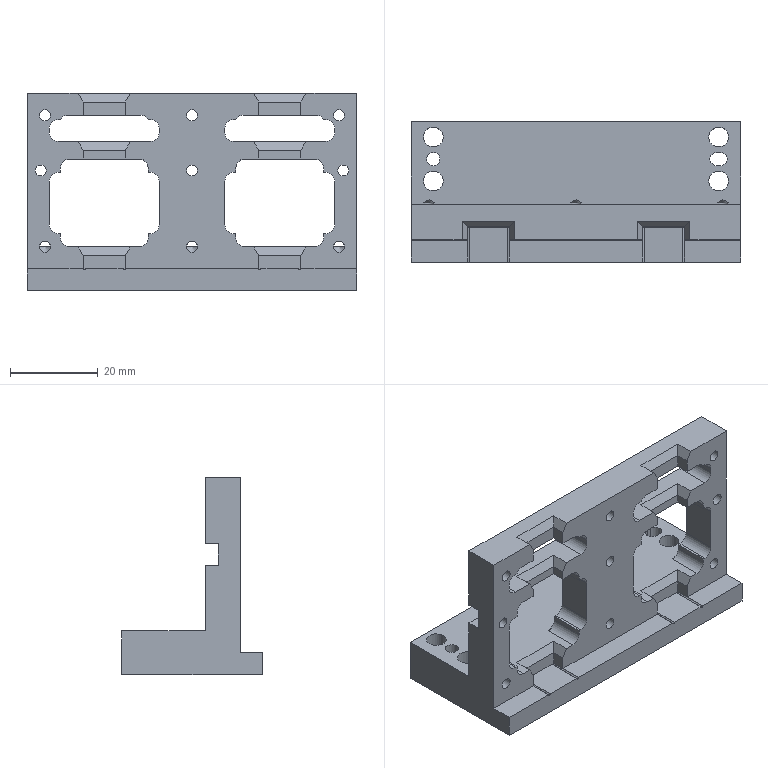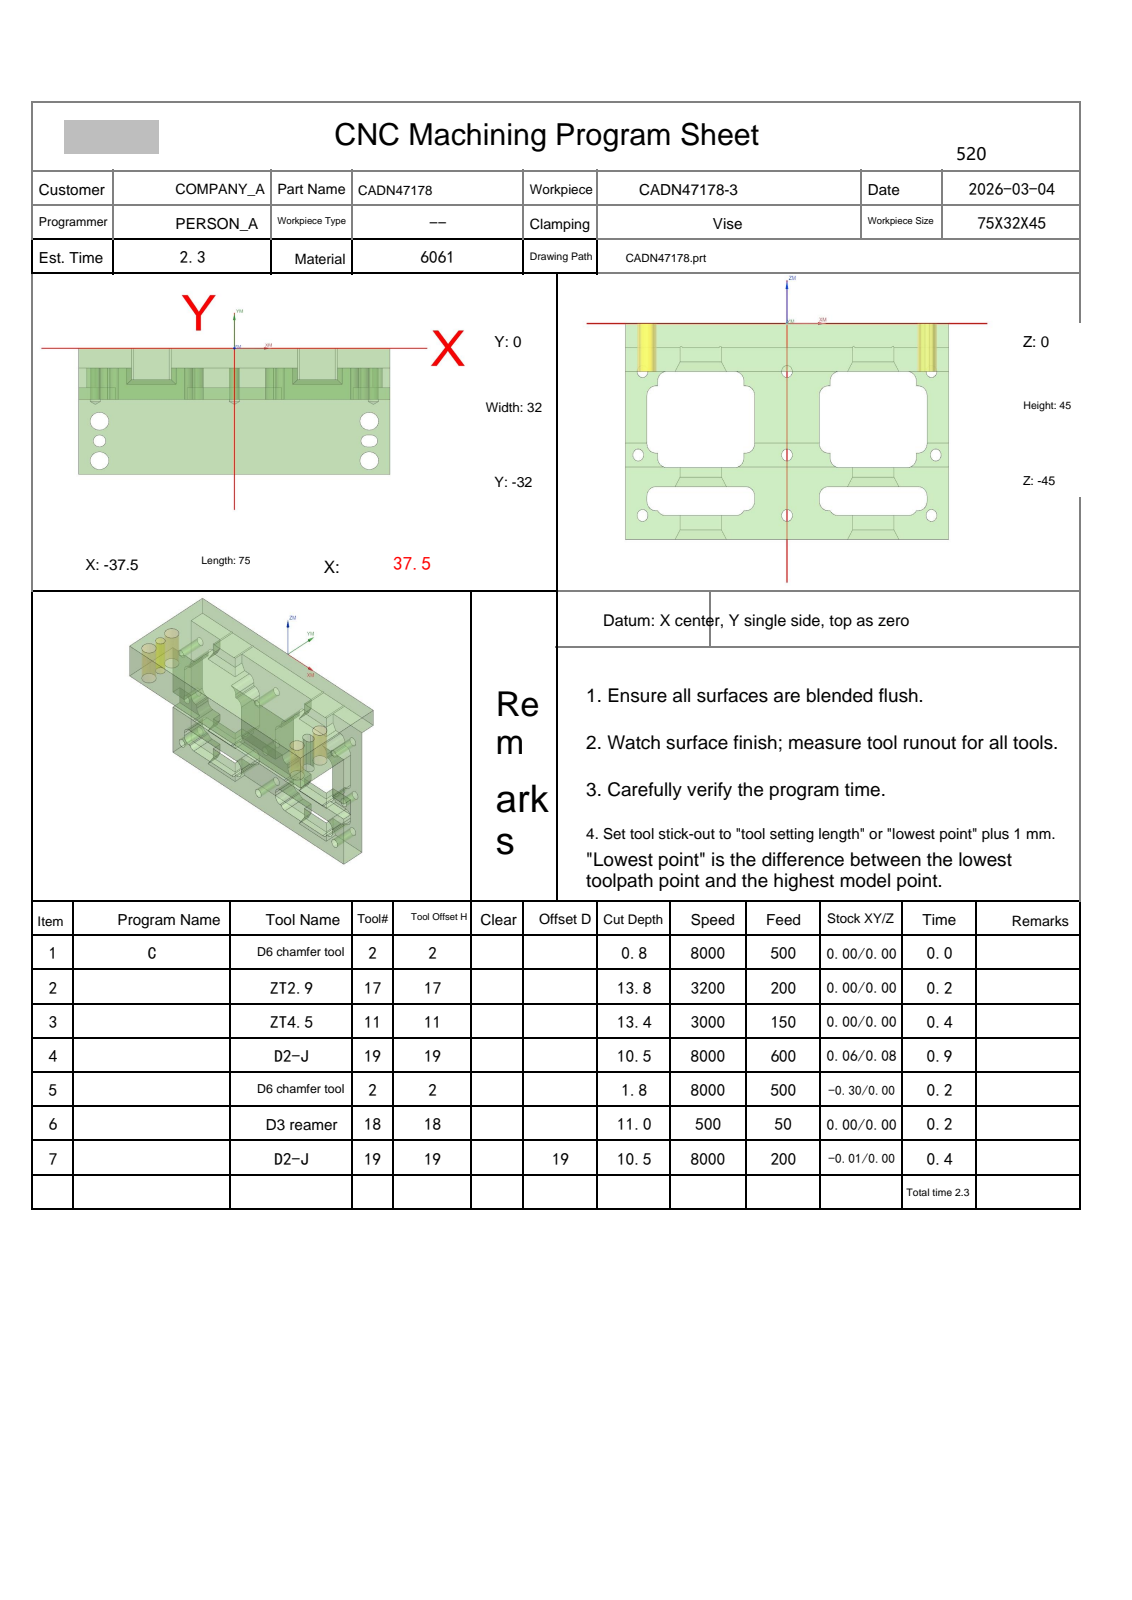NC program | NX | posted by the shop | part box 75 x 32 x 45 mm
Whole program:
%
O0001
(Machine time: 3.72 MIN)
(===Total Tool:5===)
(T2=D6 chamfer tool   D=6.   R=0.   D-  H02 Z=-1.8  )
(T17=ZT2.9  D=2.9  DR_a=120 D-  H17 Z=-13.84)
(T11=ZT4.5  D=4.5  DR_a=118 D-  H11 Z=-13.35)
(T19=D2-J   D=2.   R=0.   D-  H19 Z=-10.5 )
(T18=D3 reamer   D=3.   DR_a=180 D-  H18 Z=-11.  )
G80 G90 G17 G49 G40
G91 G28 Z0
M01
N1 T02 M06
(D6 chamfer tool  D=6. R=0. H=02 ce=0.00 di=0.00)
G00 G90 G54 X-32.5 Y-28.5 M03 S8000
G43 H02 Z30.
M08
G98 G81 X-32.5 Y-28.5 Z-.8 R1. F500.
Y-23.5
Y-18.5
X32.5
Y-28.5
G80
G00 Z30.
G00 G90 X32. Y-23.5 M03 S8000
Z30.
G98 G81 X32. Y-23.5 Z-.8 R1. F500.
G80
G00 Z30.
G91 G28 Z0.0
M05
M09
G91 G28 Z0.0
M01
N2 T17 M06
(ZT2.9 D=2.9 DR_a=120 H=17)
G00 G90 G54 X-32.5 Y-23.5 M03 S3200
G43 H17 Z30.
M08
G98 G83 X-32.5 Y-23.5 Z-13.837 R1. F200. Q2.
G80
G00 Z30.
G00 G90 X32. Y-23.5 M03 S3200
Z30.
G98 G83 X32. Y-23.5 Z-13.837 R1. F200. Q2.
G80
G00 Z30.
G91 G28 Z0.0
M05
M09
G91 G28 Z0.0
M01
N3 T11 M06
(ZT4.5 D=4.5 DR_a=118 H=11)
G00 G90 G54 X-32.5 Y-28.5 M03 S3000
G43 H11 Z30.
M08
G98 G83 X-32.5 Y-28.5 Z-13.352 R1. F150. Q3.
Y-18.5
X32.5
Y-28.5
G80
G00 Z30.
G91 G28 Z0.0
M05
M09
G91 G28 Z0.0
M01
N4 T19 M06
(D2-J  D=2. R=0. H=19 ce=0.06 di=0.08)
G00 G90 G54 X31.56 Y-23.583 M03 S8000
G43 H19 Z30.
M08
Z.8
G01 Y-23.665 Z.796 F600.
X31.835 Y-23.94 Z.775
X33.165 Z.706
X33.44 Y-23.665 Z.685
Y-23.335 Z.668
X33.165 Y-23.06 Z.648
X31.835 Z.578
X31.56 Y-23.335 Z.557
Y-23.665 Z.54
X31.835 Y-23.94 Z.52
X33.165 Z.45
X33.44 Y-23.665 Z.43
Y-23.335 Z.412
X33.165 Y-23.06 Z.392
X31.835 Z.322
X31.56 Y-23.335 Z.302
Y-23.665 Z.285
X31.835 Y-23.94 Z.264
X33.165 Z.194
X33.44 Y-23.665 Z.174
Y-23.335 Z.157
X33.165 Y-23.06 Z.136
X31.835 Z.067
X31.56 Y-23.335 Z.046
Y-23.665 Z.029
X31.835 Y-23.94 Z.009
X32. Z0.0
X33. Z-.021
G03 X33.44 Y-23.5 Z-.035 I0.0 J.44
X33. Y-23.06 Z-.05 I-.44 J0.0
G01 X32. Z-.07
G03 X31.56 Y-23.5 Z-.085 I0.0 J-.44
X32. Y-23.94 Z-.099 I.44 J0.0
G01 X33. Z-.12
G03 X33.44 Y-23.5 Z-.134 I0.0 J.44
X33. Y-23.06 Z-.149 I-.44 J0.0
G01 X32. Z-.169
G03 X31.56 Y-23.5 Z-.184 I0.0 J-.44
X32. Y-23.94 Z-.198 I.44 J0.0
G01 X33. Z-.219
G03 X33.44 Y-23.5 Z-.233 I0.0 J.44
X33. Y-23.06 Z-.248 I-.44 J0.0
G01 X32. Z-.268
G03 X31.56 Y-23.5 Z-.283 I0.0 J-.44
X32. Y-23.94 Z-.297 I.44 J0.0
G01 X33. Z-.318
G03 X33.44 Y-23.5 Z-.332 I0.0 J.44
X33. Y-23.06 Z-.347 I-.44 J0.0
G01 X32. Z-.367
G03 X31.56 Y-23.5 Z-.382 I0.0 J-.44
X32. Y-23.94 Z-.396 I.44 J0.0
G01 X33. Z-.417
G03 X33.44 Y-23.5 Z-.431 I0.0 J.44
X33. Y-23.06 Z-.446 I-.44 J0.0
G01 X32. Z-.467
G03 X31.56 Y-23.5 Z-.481 I0.0 J-.44
X32. Y-23.94 Z-.495 I.44 J0.0
G01 X33. Z-.516
G03 X33.44 Y-23.5 Z-.53 I0.0 J.44
X33. Y-23.06 Z-.545 I-.44 J0.0
G01 X32. Z-.566
G03 X31.56 Y-23.5 Z-.58 I0.0 J-.44
X32. Y-23.94 Z-.594 I.44 J0.0
G01 X33. Z-.615
G03 X33.44 Y-23.5 Z-.629 I0.0 J.44
X33. Y-23.06 Z-.644 I-.44 J0.0
G01 X32. Z-.665
G03 X31.56 Y-23.5 Z-.679 I0.0 J-.44
X32. Y-23.94 Z-.693 I.44 J0.0
G01 X33. Z-.714
G03 X33.44 Y-23.5 Z-.729 I0.0 J.44
X33. Y-23.06 Z-.743 I-.44 J0.0
G01 X32. Z-.764
G03 X31.56 Y-23.5 Z-.778 I0.0 J-.44
X32. Y-23.94 Z-.792 I.44 J0.0
G01 X33. Z-.813
G03 X33.44 Y-23.5 Z-.828 I0.0 J.44
X33. Y-23.06 Z-.842 I-.44 J0.0
G01 X32. Z-.863
G03 X31.56 Y-23.5 Z-.877 I0.0 J-.44
X32. Y-23.94 Z-.892 I.44 J0.0
G01 X33. Z-.912
G03 X33.44 Y-23.5 Z-.927 I0.0 J.44
X33. Y-23.06 Z-.941 I-.44 J0.0
G01 X32. Z-.962
G03 X31.56 Y-23.5 Z-.976 I0.0 J-.44
X32. Y-23.94 Z-.991 I.44 J0.0
G01 X33. Z-1.011
G03 X33.44 Y-23.5 Z-1.026 I0.0 J.44
X33. Y-23.06 Z-1.04 I-.44 J0.0
G01 X32. Z-1.061
G03 X31.56 Y-23.5 Z-1.075 I0.0 J-.44
X32. Y-23.94 Z-1.09 I.44 J0.0
G01 X33. Z-1.11
G03 X33.44 Y-23.5 Z-1.125 I0.0 J.44
X33. Y-23.06 Z-1.139 I-.44 J0.0
G01 X32. Z-1.16
G03 X31.56 Y-23.5 Z-1.174 I0.0 J-.44
X32. Y-23.94 Z-1.189 I.44 J0.0
G01 X33. Z-1.209
G03 X33.44 Y-23.5 Z-1.224 I0.0 J.44
X33. Y-23.06 Z-1.238 I-.44 J0.0
G01 X32. Z-1.259
G03 X31.56 Y-23.5 Z-1.273 I0.0 J-.44
X32. Y-23.94 Z-1.288 I.44 J0.0
G01 X33. Z-1.309
G03 X33.44 Y-23.5 Z-1.323 I0.0 J.44
X33. Y-23.06 Z-1.337 I-.44 J0.0
G01 X32. Z-1.358
G03 X31.56 Y-23.5 Z-1.372 I0.0 J-.44
X32. Y-23.94 Z-1.387 I.44 J0.0
G01 X33. Z-1.408
G03 X33.44 Y-23.5 Z-1.422 I0.0 J.44
X33. Y-23.06 Z-1.436 I-.44 J0.0
G01 X32. Z-1.457
G03 X31.56 Y-23.5 Z-1.471 I0.0 J-.44
X32. Y-23.94 Z-1.486 I.44 J0.0
G01 X33. Z-1.507
G03 X33.44 Y-23.5 Z-1.521 I0.0 J.44
X33. Y-23.06 Z-1.535 I-.44 J0.0
G01 X32. Z-1.556
G03 X31.56 Y-23.5 Z-1.571 I0.0 J-.44
X32. Y-23.94 Z-1.585 I.44 J0.0
G01 X33. Z-1.606
G03 X33.44 Y-23.5 Z-1.62 I0.0 J.44
X33. Y-23.06 Z-1.634 I-.44 J0.0
G01 X32. Z-1.655
G03 X31.56 Y-23.5 Z-1.67 I0.0 J-.44
X32. Y-23.94 Z-1.684 I.44 J0.0
G01 X33. Z-1.705
G03 X33.44 Y-23.5 Z-1.719 I0.0 J.44
X33. Y-23.06 Z-1.733 I-.44 J0.0
G01 X32. Z-1.754
G03 X31.56 Y-23.5 Z-1.769 I0.0 J-.44
X32. Y-23.94 Z-1.783 I.44 J0.0
G01 X33. Z-1.804
G03 X33.44 Y-23.5 Z-1.818 I0.0 J.44
X33. Y-23.06 Z-1.833 I-.44 J0.0
G01 X32. Z-1.853
G03 X31.56 Y-23.5 Z-1.868 I0.0 J-.44
X32. Y-23.94 Z-1.882 I.44 J0.0
G01 X33. Z-1.903
G03 X33.44 Y-23.5 Z-1.917 I0.0 J.44
X33. Y-23.06 Z-1.932 I-.44 J0.0
G01 X32. Z-1.952
G03 X31.56 Y-23.5 Z-1.967 I0.0 J-.44
X32. Y-23.94 Z-1.981 I.44 J0.0
G01 X33. Z-2.002
G03 X33.44 Y-23.5 Z-2.016 I0.0 J.44
X33. Y-23.06 Z-2.031 I-.44 J0.0
G01 X32. Z-2.051
G03 X31.56 Y-23.5 Z-2.066 I0.0 J-.44
X32. Y-23.94 Z-2.08 I.44 J0.0
G01 X33. Z-2.101
G03 X33.44 Y-23.5 Z-2.115 I0.0 J.44
X33. Y-23.06 Z-2.13 I-.44 J0.0
G01 X32. Z-2.151
G03 X31.56 Y-23.5 Z-2.165 I0.0 J-.44
X32. Y-23.94 Z-2.179 I.44 J0.0
G01 X33. Z-2.2
G03 X33.44 Y-23.5 Z-2.214 I0.0 J.44
X33. Y-23.06 Z-2.229 I-.44 J0.0
G01 X32. Z-2.25
G03 X31.56 Y-23.5 Z-2.264 I0.0 J-.44
X32. Y-23.94 Z-2.278 I.44 J0.0
G01 X33. Z-2.299
G03 X33.44 Y-23.5 Z-2.313 I0.0 J.44
X33. Y-23.06 Z-2.328 I-.44 J0.0
G01 X32. Z-2.349
G03 X31.56 Y-23.5 Z-2.363 I0.0 J-.44
X32. Y-23.94 Z-2.377 I.44 J0.0
G01 X33. Z-2.398
G03 X33.44 Y-23.5 Z-2.413 I0.0 J.44
X33. Y-23.06 Z-2.427 I-.44 J0.0
G01 X32. Z-2.448
G03 X31.56 Y-23.5 Z-2.462 I0.0 J-.44
X32. Y-23.94 Z-2.476 I.44 J0.0
G01 X33. Z-2.497
G03 X33.44 Y-23.5 Z-2.512 I0.0 J.44
X33. Y-23.06 Z-2.526 I-.44 J0.0
G01 X32. Z-2.547
G03 X31.56 Y-23.5 Z-2.561 I0.0 J-.44
X32. Y-23.94 Z-2.575 I.44 J0.0
G01 X33. Z-2.596
G03 X33.44 Y-23.5 Z-2.611 I0.0 J.44
X33. Y-23.06 Z-2.625 I-.44 J0.0
G01 X32. Z-2.646
G03 X31.56 Y-23.5 Z-2.66 I0.0 J-.44
X32. Y-23.94 Z-2.675 I.44 J0.0
G01 X33. Z-2.695
G03 X33.44 Y-23.5 Z-2.71 I0.0 J.44
X33. Y-23.06 Z-2.724 I-.44 J0.0
G01 X32. Z-2.745
G03 X31.56 Y-23.5 Z-2.759 I0.0 J-.44
X32. Y-23.94 Z-2.774 I.44 J0.0
G01 X33. Z-2.794
G03 X33.44 Y-23.5 Z-2.809 I0.0 J.44
X33. Y-23.06 Z-2.823 I-.44 J0.0
G01 X32. Z-2.844
G03 X31.56 Y-23.5 Z-2.858 I0.0 J-.44
X32. Y-23.94 Z-2.873 I.44 J0.0
G01 X33. Z-2.893
G03 X33.44 Y-23.5 Z-2.908 I0.0 J.44
X33. Y-23.06 Z-2.922 I-.44 J0.0
G01 X32. Z-2.943
G03 X31.56 Y-23.5 Z-2.957 I0.0 J-.44
X32. Y-23.94 Z-2.972 I.44 J0.0
G01 X33. Z-2.992
G03 X33.44 Y-23.5 Z-3.007 I0.0 J.44
X33. Y-23.06 Z-3.021 I-.44 J0.0
G01 X32. Z-3.042
G03 X31.56 Y-23.5 Z-3.056 I0.0 J-.44
X32. Y-23.94 Z-3.071 I.44 J0.0
G01 X33. Z-3.092
G03 X33.44 Y-23.5 Z-3.106 I0.0 J.44
X33. Y-23.06 Z-3.12 I-.44 J0.0
G01 X32. Z-3.141
G03 X31.56 Y-23.5 Z-3.155 I0.0 J-.44
X32. Y-23.94 Z-3.17 I.44 J0.0
G01 X33. Z-3.191
G03 X33.44 Y-23.5 Z-3.205 I0.0 J.44
X33. Y-23.06 Z-3.219 I-.44 J0.0
G01 X32. Z-3.24
G03 X31.56 Y-23.5 Z-3.254 I0.0 J-.44
X32. Y-23.94 Z-3.269 I.44 J0.0
G01 X33. Z-3.29
G03 X33.44 Y-23.5 Z-3.304 I0.0 J.44
X33. Y-23.06 Z-3.318 I-.44 J0.0
G01 X32. Z-3.339
G03 X31.56 Y-23.5 Z-3.354 I0.0 J-.44
X32. Y-23.94 Z-3.368 I.44 J0.0
G01 X33. Z-3.389
G03 X33.44 Y-23.5 Z-3.403 I0.0 J.44
X33. Y-23.06 Z-3.417 I-.44 J0.0
G01 X32. Z-3.438
G03 X31.56 Y-23.5 Z-3.453 I0.0 J-.44
X32. Y-23.94 Z-3.467 I.44 J0.0
G01 X33. Z-3.488
G03 X33.44 Y-23.5 Z-3.502 I0.0 J.44
X33. Y-23.06 Z-3.517 I-.44 J0.0
G01 X32. Z-3.537
G03 X31.56 Y-23.5 Z-3.552 I0.0 J-.44
X32. Y-23.94 Z-3.566 I.44 J0.0
G01 X33. Z-3.587
G03 X33.44 Y-23.5 Z-3.601 I0.0 J.44
X33. Y-23.06 Z-3.616 I-.44 J0.0
G01 X32. Z-3.636
G03 X31.56 Y-23.5 Z-3.651 I0.0 J-.44
X32. Y-23.94 Z-3.665 I.44 J0.0
G01 X33. Z-3.686
G03 X33.44 Y-23.5 Z-3.7 I0.0 J.44
X33. Y-23.06 Z-3.715 I-.44 J0.0
G01 X32. Z-3.735
G03 X31.56 Y-23.5 Z-3.75 I0.0 J-.44
X32. Y-23.94 Z-3.764 I.44 J0.0
G01 X33. Z-3.785
G03 X33.44 Y-23.5 Z-3.799 I0.0 J.44
X33. Y-23.06 Z-3.814 I-.44 J0.0
G01 X32. Z-3.834
G03 X31.56 Y-23.5 Z-3.849 I0.0 J-.44
X32. Y-23.94 Z-3.863 I.44 J0.0
G01 X33. Z-3.884
G03 X33.44 Y-23.5 Z-3.898 I0.0 J.44
X33. Y-23.06 Z-3.913 I-.44 J0.0
G01 X32. Z-3.934
G03 X31.56 Y-23.5 Z-3.948 I0.0 J-.44
X32. Y-23.94 Z-3.962 I.44 J0.0
G01 X33. Z-3.983
G03 X33.44 Y-23.5 Z-3.997 I0.0 J.44
X33. Y-23.06 Z-4.012 I-.44 J0.0
G01 X32. Z-4.033
G03 X31.56 Y-23.5 Z-4.047 I0.0 J-.44
X32. Y-23.94 Z-4.061 I.44 J0.0
G01 X33. Z-4.082
G03 X33.44 Y-23.5 Z-4.096 I0.0 J.44
X33. Y-23.06 Z-4.111 I-.44 J0.0
G01 X32. Z-4.132
G03 X31.56 Y-23.5 Z-4.146 I0.0 J-.44
X32. Y-23.94 Z-4.16 I.44 J0.0
G01 X33. Z-4.181
G03 X33.44 Y-23.5 Z-4.196 I0.0 J.44
X33. Y-23.06 Z-4.21 I-.44 J0.0
G01 X32. Z-4.231
G03 X31.56 Y-23.5 Z-4.245 I0.0 J-.44
X32. Y-23.94 Z-4.259 I.44 J0.0
G01 X33. Z-4.28
G03 X33.44 Y-23.5 Z-4.295 I0.0 J.44
X33. Y-23.06 Z-4.309 I-.44 J0.0
G01 X32. Z-4.33
G03 X31.56 Y-23.5 Z-4.344 I0.0 J-.44
X32. Y-23.94 Z-4.358 I.44 J0.0
G01 X33. Z-4.379
G03 X33.44 Y-23.5 Z-4.394 I0.0 J.44
X33. Y-23.06 Z-4.408 I-.44 J0.0
G01 X32. Z-4.429
G03 X31.56 Y-23.5 Z-4.443 I0.0 J-.44
X32. Y-23.94 Z-4.458 I.44 J0.0
G01 X33. Z-4.478
G03 X33.44 Y-23.5 Z-4.493 I0.0 J.44
X33. Y-23.06 Z-4.507 I-.44 J0.0
G01 X32. Z-4.528
G03 X31.56 Y-23.5 Z-4.542 I0.0 J-.44
X32. Y-23.94 Z-4.557 I.44 J0.0
G01 X33. Z-4.577
G03 X33.44 Y-23.5 Z-4.592 I0.0 J.44
X33. Y-23.06 Z-4.606 I-.44 J0.0
G01 X32. Z-4.627
G03 X31.56 Y-23.5 Z-4.641 I0.0 J-.44
X32. Y-23.94 Z-4.656 I.44 J0.0
G01 X33. Z-4.676
G03 X33.44 Y-23.5 Z-4.691 I0.0 J.44
X33. Y-23.06 Z-4.705 I-.44 J0.0
G01 X32. Z-4.726
G03 X31.56 Y-23.5 Z-4.74 I0.0 J-.44
X32. Y-23.94 Z-4.755 I.44 J0.0
G01 X33. Z-4.776
G03 X33.44 Y-23.5 Z-4.79 I0.0 J.44
X33. Y-23.06 Z-4.804 I-.44 J0.0
G01 X32. Z-4.825
G03 X31.56 Y-23.5 Z-4.839 I0.0 J-.44
X32. Y-23.94 Z-4.854 I.44 J0.0
G01 X33. Z-4.875
G03 X33.44 Y-23.5 Z-4.889 I0.0 J.44
X33. Y-23.06 Z-4.903 I-.44 J0.0
G01 X32. Z-4.924
G03 X31.56 Y-23.5 Z-4.938 I0.0 J-.44
X32. Y-23.94 Z-4.953 I.44 J0.0
G01 X33. Z-4.974
G03 X33.44 Y-23.5 Z-4.988 I0.0 J.44
X33. Y-23.06 Z-5.002 I-.44 J0.0
G01 X32. Z-5.023
G03 X31.56 Y-23.5 Z-5.038 I0.0 J-.44
X32. Y-23.94 Z-5.052 I.44 J0.0
G01 X33. Z-5.073
G03 X33.44 Y-23.5 Z-5.087 I0.0 J.44
X33. Y-23.06 Z-5.101 I-.44 J0.0
G01 X32. Z-5.122
G03 X31.56 Y-23.5 Z-5.137 I0.0 J-.44
X32. Y-23.94 Z-5.151 I.44 J0.0
G01 X33. Z-5.172
G03 X33.44 Y-23.5 Z-5.186 I0.0 J.44
X33. Y-23.06 Z-5.2 I-.44 J0.0
G01 X32. Z-5.221
G03 X31.56 Y-23.5 Z-5.236 I0.0 J-.44
X32. Y-23.94 Z-5.25 I.44 J0.0
G01 X33. Z-5.271
G03 X33.44 Y-23.5 Z-5.285 I0.0 J.44
X33. Y-23.06 Z-5.3 I-.44 J0.0
G01 X32. Z-5.32
G03 X31.56 Y-23.5 Z-5.335 I0.0 J-.44
X32. Y-23.94 Z-5.349 I.44 J0.0
G01 X33. Z-5.37
G03 X33.44 Y-23.5 Z-5.384 I0.0 J.44
X33. Y-23.06 Z-5.399 I-.44 J0.0
G01 X32. Z-5.419
G03 X31.56 Y-23.5 Z-5.434 I0.0 J-.44
X32. Y-23.94 Z-5.448 I.44 J0.0
G01 X33. Z-5.469
G03 X33.44 Y-23.5 Z-5.483 I0.0 J.44
X33. Y-23.06 Z-5.498 I-.44 J0.0
G01 X32. Z-5.518
G03 X31.56 Y-23.5 Z-5.533 I0.0 J-.44
X32. Y-23.94 Z-5.547 I.44 J0.0
G01 X33. Z-5.568
G03 X33.44 Y-23.5 Z-5.582 I0.0 J.44
X33. Y-23.06 Z-5.597 I-.44 J0.0
G01 X32. Z-5.617
G03 X31.56 Y-23.5 Z-5.632 I0.0 J-.44
X32. Y-23.94 Z-5.646 I.44 J0.0
G01 X33. Z-5.667
G03 X33.44 Y-23.5 Z-5.681 I0.0 J.44
X33. Y-23.06 Z-5.696 I-.44 J0.0
G01 X32. Z-5.717
G03 X31.56 Y-23.5 Z-5.731 I0.0 J-.44
X32. Y-23.94 Z-5.745 I.44 J0.0
G01 X33. Z-5.766
G03 X33.44 Y-23.5 Z-5.78 I0.0 J.44
X33. Y-23.06 Z-5.795 I-.44 J0.0
G01 X32. Z-5.816
G03 X31.56 Y-23.5 Z-5.83 I0.0 J-.44
X32. Y-23.94 Z-5.844 I.44 J0.0
G01 X33. Z-5.865
G03 X33.44 Y-23.5 Z-5.879 I0.0 J.44
X33. Y-23.06 Z-5.894 I-.44 J0.0
G01 X32. Z-5.915
G03 X31.56 Y-23.5 Z-5.929 I0.0 J-.44
X32. Y-23.94 Z-5.943 I.44 J0.0
G01 X33. Z-5.964
G03 X33.44 Y-23.5 Z-5.979 I0.0 J.44
X33. Y-23.06 Z-5.993 I-.44 J0.0
G01 X32. Z-6.014
G03 X31.56 Y-23.5 Z-6.028 I0.0 J-.44
X32. Y-23.94 Z-6.042 I.44 J0.0
G01 X33. Z-6.063
G03 X33.44 Y-23.5 Z-6.078 I0.0 J.44
X33. Y-23.06 Z-6.092 I-.44 J0.0
G01 X32. Z-6.113
G03 X31.56 Y-23.5 Z-6.127 I0.0 J-.44
X32. Y-23.94 Z-6.142 I.44 J0.0
G01 X33. Z-6.162
G03 X33.44 Y-23.5 Z-6.177 I0.0 J.44
X33. Y-23.06 Z-6.191 I-.44 J0.0
G01 X32. Z-6.212
G03 X31.56 Y-23.5 Z-6.226 I0.0 J-.44
X32. Y-23.94 Z-6.241 I.44 J0.0
G01 X33. Z-6.261
G03 X33.44 Y-23.5 Z-6.276 I0.0 J.44
X33. Y-23.06 Z-6.29 I-.44 J0.0
G01 X32. Z-6.311
G03 X31.56 Y-23.5 Z-6.325 I0.0 J-.44
X32. Y-23.94 Z-6.34 I.44 J0.0
G01 X33. Z-6.36
G03 X33.44 Y-23.5 Z-6.375 I0.0 J.44
X33. Y-23.06 Z-6.389 I-.44 J0.0
G01 X32. Z-6.41
G03 X31.56 Y-23.5 Z-6.424 I0.0 J-.44
X32. Y-23.94 Z-6.439 I.44 J0.0
G01 X33. Z-6.459
G03 X33.44 Y-23.5 Z-6.474 I0.0 J.44
X33. Y-23.06 Z-6.488 I-.44 J0.0
G01 X32. Z-6.509
G03 X31.56 Y-23.5 Z-6.523 I0.0 J-.44
X32. Y-23.94 Z-6.538 I.44 J0.0
G01 X33. Z-6.559
G03 X33.44 Y-23.5 Z-6.573 I0.0 J.44
X33. Y-23.06 Z-6.587 I-.44 J0.0
G01 X32. Z-6.608
G03 X31.56 Y-23.5 Z-6.622 I0.0 J-.44
X32. Y-23.94 Z-6.637 I.44 J0.0
G01 X33. Z-6.658
G03 X33.44 Y-23.5 Z-6.672 I0.0 J.44
X33. Y-23.06 Z-6.686 I-.44 J0.0
G01 X32. Z-6.707
G03 X31.56 Y-23.5 Z-6.721 I0.0 J-.44
X32. Y-23.94 Z-6.736 I.44 J0.0
G01 X33. Z-6.757
G03 X33.44 Y-23.5 Z-6.771 I0.0 J.44
X33. Y-23.06 Z-6.785 I-.44 J0.0
G01 X32. Z-6.806
G03 X31.56 Y-23.5 Z-6.821 I0.0 J-.44
X32. Y-23.94 Z-6.835 I.44 J0.0
G01 X33. Z-6.856
G03 X33.44 Y-23.5 Z-6.87 I0.0 J.44
X33. Y-23.06 Z-6.884 I-.44 J0.0
G01 X32. Z-6.905
G03 X31.56 Y-23.5 Z-6.92 I0.0 J-.44
X32. Y-23.94 Z-6.934 I.44 J0.0
G01 X33. Z-6.955
G03 X33.44 Y-23.5 Z-6.969 I0.0 J.44
X33. Y-23.06 Z-6.983 I-.44 J0.0
G01 X32. Z-7.004
G03 X31.56 Y-23.5 Z-7.019 I0.0 J-.44
X32. Y-23.94 Z-7.033 I.44 J0.0
G01 X33. Z-7.054
G03 X33.44 Y-23.5 Z-7.068 I0.0 J.44
X33. Y-23.06 Z-7.083 I-.44 J0.0
G01 X32. Z-7.103
G03 X31.56 Y-23.5 Z-7.118 I0.0 J-.44
X32. Y-23.94 Z-7.132 I.44 J0.0
G01 X33. Z-7.153
G03 X33.44 Y-23.5 Z-7.167 I0.0 J.44
X33. Y-23.06 Z-7.182 I-.44 J0.0
G01 X32. Z-7.202
G03 X31.56 Y-23.5 Z-7.217 I0.0 J-.44
X32. Y-23.94 Z-7.231 I.44 J0.0
G01 X33. Z-7.252
G03 X33.44 Y-23.5 Z-7.266 I0.0 J.44
X33. Y-23.06 Z-7.281 I-.44 J0.0
G01 X32. Z-7.301
G03 X31.56 Y-23.5 Z-7.316 I0.0 J-.44
X32. Y-23.94 Z-7.33 I.44 J0.0
G01 X33. Z-7.351
G03 X33.44 Y-23.5 Z-7.365 I0.0 J.44
X33. Y-23.06 Z-7.38 I-.44 J0.0
G01 X32. Z-7.401
G03 X31.56 Y-23.5 Z-7.415 I0.0 J-.44
X32. Y-23.94 Z-7.429 I.44 J0.0
G01 X33. Z-7.45
G03 X33.44 Y-23.5 Z-7.464 I0.0 J.44
X33. Y-23.06 Z-7.479 I-.44 J0.0
G01 X32. Z-7.5
G03 X31.56 Y-23.5 Z-7.514 I0.0 J-.44
X32. Y-23.94 Z-7.528 I.44 J0.0
G01 X33. Z-7.549
G03 X33.44 Y-23.5 Z-7.563 I0.0 J.44
X33. Y-23.06 Z-7.578 I-.44 J0.0
G01 X32. Z-7.599
G03 X31.56 Y-23.5 Z-7.613 I0.0 J-.44
X32. Y-23.94 Z-7.627 I.44 J0.0
G01 X33. Z-7.648
G03 X33.44 Y-23.5 Z-7.663 I0.0 J.44
X33. Y-23.06 Z-7.677 I-.44 J0.0
G01 X32. Z-7.698
G03 X31.56 Y-23.5 Z-7.712 I0.0 J-.44
X32. Y-23.94 Z-7.726 I.44 J0.0
G01 X33. Z-7.747
G03 X33.44 Y-23.5 Z-7.762 I0.0 J.44
X33. Y-23.06 Z-7.776 I-.44 J0.0
G01 X32. Z-7.797
G03 X31.56 Y-23.5 Z-7.811 I0.0 J-.44
X32. Y-23.94 Z-7.825 I.44 J0.0
G01 X33. Z-7.846
G03 X33.44 Y-23.5 Z-7.861 I0.0 J.44
X33. Y-23.06 Z-7.875 I-.44 J0.0
G01 X32. Z-7.896
G03 X31.56 Y-23.5 Z-7.91 I0.0 J-.44
X32. Y-23.94 Z-7.925 I.44 J0.0
G01 X33. Z-7.945
G03 X33.44 Y-23.5 Z-7.96 I0.0 J.44
X33. Y-23.06 Z-7.974 I-.44 J0.0
G01 X32. Z-7.995
G03 X31.56 Y-23.5 Z-8.009 I0.0 J-.44
X32. Y-23.94 Z-8.024 I.44 J0.0
G01 X33. Z-8.044
G03 X33.44 Y-23.5 Z-8.059 I0.0 J.44
X33. Y-23.06 Z-8.073 I-.44 J0.0
G01 X32. Z-8.094
G03 X31.56 Y-23.5 Z-8.108 I0.0 J-.44
X32. Y-23.94 Z-8.123 I.44 J0.0
G01 X33. Z-8.143
G03 X33.44 Y-23.5 Z-8.158 I0.0 J.44
X33. Y-23.06 Z-8.172 I-.44 J0.0
G01 X32. Z-8.193
G03 X31.56 Y-23.5 Z-8.207 I0.0 J-.44
X32. Y-23.94 Z-8.222 I.44 J0.0
G01 X33. Z-8.242
G03 X33.44 Y-23.5 Z-8.257 I0.0 J.44
X33. Y-23.06 Z-8.271 I-.44 J0.0
G01 X32. Z-8.292
G03 X31.56 Y-23.5 Z-8.306 I0.0 J-.44
X32. Y-23.94 Z-8.321 I.44 J0.0
G01 X33. Z-8.342
G03 X33.44 Y-23.5 Z-8.356 I0.0 J.44
X33. Y-23.06 Z-8.37 I-.44 J0.0
G01 X32. Z-8.391
G03 X31.56 Y-23.5 Z-8.405 I0.0 J-.44
X32. Y-23.94 Z-8.42 I.44 J0.0
G01 X33. Z-8.441
G03 X33.44 Y-23.5 Z-8.455 I0.0 J.44
X33. Y-23.06 Z-8.469 I-.44 J0.0
G01 X32. Z-8.49
G03 X31.56 Y-23.5 Z-8.504 I0.0 J-.44
X32. Y-23.94 Z-8.519 I.44 J0.0
G01 X33. Z-8.54
G03 X33.44 Y-23.5 Z-8.554 I0.0 J.44
X33. Y-23.06 Z-8.568 I-.44 J0.0
G01 X32. Z-8.589
G03 X31.56 Y-23.5 Z-8.604 I0.0 J-.44
X32. Y-23.94 Z-8.618 I.44 J0.0
G01 X33. Z-8.639
G03 X33.44 Y-23.5 Z-8.653 I0.0 J.44
X33. Y-23.06 Z-8.667 I-.44 J0.0
G01 X32. Z-8.688
G03 X31.56 Y-23.5 Z-8.703 I0.0 J-.44
X32. Y-23.94 Z-8.717 I.44 J0.0
G01 X33. Z-8.738
G03 X33.44 Y-23.5 Z-8.752 I0.0 J.44
X33. Y-23.06 Z-8.767 I-.44 J0.0
G01 X32. Z-8.787
G03 X31.56 Y-23.5 Z-8.802 I0.0 J-.44
X32. Y-23.94 Z-8.816 I.44 J0.0
G01 X33. Z-8.837
G03 X33.44 Y-23.5 Z-8.851 I0.0 J.44
X33. Y-23.06 Z-8.866 I-.44 J0.0
G01 X32. Z-8.886
G03 X31.56 Y-23.5 Z-8.901 I0.0 J-.44
X32. Y-23.94 Z-8.915 I.44 J0.0
G01 X33. Z-8.936
G03 X33.44 Y-23.5 Z-8.95 I0.0 J.44
X33. Y-23.06 Z-8.965 I-.44 J0.0
G01 X32. Z-8.985
G03 X31.56 Y-23.5 Z-9. I0.0 J-.44
X32. Y-23.94 Z-9.014 I.44 J0.0
G01 X33. Z-9.035
G03 X33.44 Y-23.5 Z-9.049 I0.0 J.44
X33. Y-23.06 Z-9.064 I-.44 J0.0
G01 X32. Z-9.084
G03 X31.56 Y-23.5 Z-9.099 I0.0 J-.44
X32. Y-23.94 Z-9.113 I.44 J0.0
G01 X33. Z-9.134
G03 X33.44 Y-23.5 Z-9.148 I0.0 J.44
X33. Y-23.06 Z-9.163 I-.44 J0.0
G01 X32. Z-9.184
G03 X31.56 Y-23.5 Z-9.198 I0.0 J-.44
X32. Y-23.94 Z-9.212 I.44 J0.0
G01 X33. Z-9.233
G03 X33.44 Y-23.5 Z-9.247 I0.0 J.44
X33. Y-23.06 Z-9.262 I-.44 J0.0
G01 X32. Z-9.283
G03 X31.56 Y-23.5 Z-9.297 I0.0 J-.44
X32. Y-23.94 Z-9.311 I.44 J0.0
G01 X33. Z-9.332
G03 X33.44 Y-23.5 Z-9.346 I0.0 J.44
X33. Y-23.06 Z-9.361 I-.44 J0.0
G01 X32. Z-9.382
G03 X31.56 Y-23.5 Z-9.396 I0.0 J-.44
X32. Y-23.94 Z-9.41 I.44 J0.0
G01 X33. Z-9.431
G03 X33.44 Y-23.5 Z-9.446 I0.0 J.44
X33. Y-23.06 Z-9.46 I-.44 J0.0
G01 X32. Z-9.481
G03 X31.56 Y-23.5 Z-9.495 I0.0 J-.44
X32. Y-23.94 Z-9.509 I.44 J0.0
G01 X33. Z-9.53
G03 X33.44 Y-23.5 Z-9.545 I0.0 J.44
X33. Y-23.06 Z-9.559 I-.44 J0.0
G01 X32. Z-9.58
G03 X31.56 Y-23.5 Z-9.594 I0.0 J-.44
X32. Y-23.94 Z-9.608 I.44 J0.0
G01 X33. Z-9.629
G03 X33.44 Y-23.5 Z-9.644 I0.0 J.44
X33. Y-23.06 Z-9.658 I-.44 J0.0
G01 X32. Z-9.679
G03 X31.56 Y-23.5 Z-9.693 I0.0 J-.44
X32. Y-23.94 Z-9.708 I.44 J0.0
G01 X33. Z-9.728
G03 X33.44 Y-23.5 Z-9.743 I0.0 J.44
X33. Y-23.06 Z-9.757 I-.44 J0.0
G01 X32. Z-9.778
G03 X31.56 Y-23.5 Z-9.792 I0.0 J-.44
X32. Y-23.94 Z-9.807 I.44 J0.0
G01 X33. Z-9.827
G03 X33.44 Y-23.5 Z-9.842 I0.0 J.44
X33. Y-23.06 Z-9.856 I-.44 J0.0
G01 X32. Z-9.877
G03 X31.56 Y-23.5 Z-9.891 I0.0 J-.44
X32. Y-23.94 Z-9.906 I.44 J0.0
G01 X33. Z-9.926
G03 X33.44 Y-23.5 Z-9.941 I0.0 J.44
X33. Y-23.06 Z-9.955 I-.44 J0.0
G01 X32. Z-9.976
G03 X31.56 Y-23.5 Z-9.99 I0.0 J-.44
X32. Y-23.94 Z-10.005 I.44 J0.0
G01 X33. Z-10.026
G03 X33.44 Y-23.5 Z-10.04 I0.0 J.44
X33. Y-23.06 Z-10.054 I-.44 J0.0
G01 X32. Z-10.075
G03 X31.56 Y-23.5 Z-10.089 I0.0 J-.44
X32. Y-23.94 Z-10.104 I.44 J0.0
G01 X33. Z-10.125
G03 X33.44 Y-23.5 Z-10.139 I0.0 J.44
X33. Y-23.06 Z-10.153 I-.44 J0.0
G01 X32. Z-10.174
G03 X31.56 Y-23.5 Z-10.188 I0.0 J-.44
X32. Y-23.94 Z-10.203 I.44 J0.0
G01 X33. Z-10.224
G03 X33.44 Y-23.5 Z-10.238 I0.0 J.44
X33. Y-23.06 Z-10.252 I-.44 J0.0
G01 X32. Z-10.273
G03 X31.56 Y-23.5 Z-10.288 I0.0 J-.44
X32. Y-23.94 Z-10.302 I.44 J0.0
G01 X33. Z-10.323
G03 X33.44 Y-23.5 Z-10.337 I0.0 J.44
X33. Y-23.06 Z-10.351 I-.44 J0.0
G01 X32. Z-10.372
G03 X31.56 Y-23.5 Z-10.387 I0.0 J-.44
X32. Y-23.94 Z-10.401 I.44 J0.0
G01 X33. Z-10.422
G03 X33.44 Y-23.5 Z-10.436 I0.0 J.44
X33. Y-23.06 Z-10.45 I-.44 J0.0
G01 X32. Z-10.471
G03 X31.56 Y-23.5 Z-10.486 I0.0 J-.44
X32. Y-23.94 Z-10.5 I.44 J0.0
G01 X33.
G03 X33.44 Y-23.5 I0.0 J.44
X33. Y-23.06 I-.44 J0.0
G01 X32.
G03 X31.56 Y-23.5 I0.0 J-.44
X32. Y-23.94 I.44 J0.0
G01 X32.4
Z-9.7
G00 Z30.
G91 G28 Z0.0
M05
M09
G91 G28 Z0.0
M01
N5 T02 M06
(D6 chamfer tool  D=6. R=0. H=02 ce=0.00 di=0.08)
G00 G90 G54 X-32.5 Y-23.5 M03 S8000
G43 H02 Z30.
M08
G98 G81 X-32.5 Y-23.5 Z-1.8 R3. F500.
G80
G00 Z30.
G00 G90 X32.482 Y-17.95 M03 S8000
Z30.
Z-.5
G01 Z-1. F500.
X32.45 Y-17.
G03 X30.95 Y-18.5 I0.0 J-1.5
X32.5 Y-20.05 I1.55 J0.0
X34.05 Y-18.5 I0.0 J1.55
X32.5 Y-16.95 I-1.55 J0.0
X30.95 Y-18.5 I0.0 J-1.55
X32.45 Y-20. I1.5 J0.0
G01 X32.482 Y-19.05
Z-.5
G00 Z30.
Y-27.95
Z-.5
G01 Z-1.
X32.45 Y-27.
G03 X30.95 Y-28.5 I0.0 J-1.5
X32.5 Y-30.05 I1.55 J0.0
X34.05 Y-28.5 I0.0 J1.55
X32.5 Y-26.95 I-1.55 J0.0
X30.95 Y-28.5 I0.0 J-1.55
X32.45 Y-30. I1.5 J0.0
G01 X32.482 Y-29.05
Z-.5
G00 Z30.
X-32.518 Y-27.95
Z-.5
G01 Z-1.
X-32.55 Y-27.
G03 X-34.05 Y-28.5 I0.0 J-1.5
X-32.5 Y-30.05 I1.55 J0.0
X-30.95 Y-28.5 I0.0 J1.55
X-32.5 Y-26.95 I-1.55 J0.0
X-34.05 Y-28.5 I0.0 J-1.55
X-32.55 Y-30. I1.5 J0.0
G01 X-32.518 Y-29.05
Z-.5
G00 Z30.
Y-17.95
Z-.5
G01 Z-1.
X-32.55 Y-17.
G03 X-34.05 Y-18.5 I0.0 J-1.5
X-32.5 Y-20.05 I1.55 J0.0
X-30.95 Y-18.5 I0.0 J1.55
X-32.5 Y-16.95 I-1.55 J0.0
X-34.05 Y-18.5 I0.0 J-1.55
X-32.55 Y-20. I1.5 J0.0
G01 X-32.518 Y-19.05
Z-.5
G00 Z30.
G00 G90 X32.525 Y-24.15 M03 S7000
Z30.
Z2.5
G01 X33.063 Z2.304 F1500.
X33.209 Y-24.119 Z2.25
X33.344 Y-24.055 Z2.195
X33.462 Y-23.962 Z2.141
X33.555 Y-23.844 Z2.086
X33.619 Y-23.709 Z2.032
X33.65 Y-23.563 Z1.977
Y-23.437 Z1.932
X33.619 Y-23.291 Z1.877
X33.555 Y-23.156 Z1.823
X33.462 Y-23.038 Z1.768
X33.344 Y-22.945 Z1.714
X33.209 Y-22.881 Z1.659
X33.063 Y-22.85 Z1.605
X31.937 Z1.195
X31.791 Y-22.881 Z1.141
X31.656 Y-22.945 Z1.086
X31.538 Y-23.038 Z1.032
X31.445 Y-23.156 Z.977
X31.381 Y-23.291 Z.923
X31.35 Y-23.437 Z.868
Y-23.563 Z.823
X31.381 Y-23.709 Z.768
X31.445 Y-23.844 Z.714
X31.538 Y-23.962 Z.659
X31.656 Y-24.055 Z.605
X31.791 Y-24.119 Z.55
X31.937 Y-24.15 Z.496
X33.063 Z.086
X33.209 Y-24.119 Z.032
X33.344 Y-24.055 Z-.023
X33.462 Y-23.962 Z-.077
X33.555 Y-23.844 Z-.132
X33.619 Y-23.709 Z-.186
X33.65 Y-23.563 Z-.241
Y-23.437 Z-.286
X33.619 Y-23.291 Z-.341
X33.555 Y-23.156 Z-.395
X33.462 Y-23.038 Z-.45
X33.344 Y-22.945 Z-.504
X33.209 Y-22.881 Z-.559
X33.063 Y-22.85 Z-.613
X32. Z-1.
G03 X31.35 Y-23.5 I0.0 J-.65
X32. Y-24.15 I.65 J0.0
G01 X33.
G03 X33.65 Y-23.5 I0.0 J.65
X33. Y-22.85 I-.65 J0.0
G01 X32.
G03 X31.548 Y-23.033 I0.0 J-.65
G01 Z1.5
G00 Z30.
G91 G28 Z0.0
M05
M09
G91 G28 Z0.0
M01
N6 T18 M06
(D3 reamer D=3. DR_a=180 H=18)
G00 G90 G54 X-32.5 Y-23.5 M03 S500
G43 H18 Z30.
M08
G98 G81 X-32.5 Y-23.5 Z-11. R1. F50.
G80
G00 Z30.
G91 G28 Z0.0
M05
M09
G91 G28 Z0.0
M01
N7 T19 M06
(D2-J  D=2. R=0. H=19 ce=-0.01 di=0.00)
G00 G90 G54 X32.132 Y-22.99 M03 S8000
G43 H19 Z30.
M08
Z.5
G01 X31.928 Z.489 F200.
X31.826 Y-23.015 Z.484
X31.731 Y-23.061 Z.478
X31.621 Y-23.152 Z.471
X31.534 Y-23.28 Z.463
X31.49 Y-23.428 Z.455
Y-23.572 Z.447
X31.539 Y-23.73 Z.438
X31.636 Y-23.864 Z.43
X31.77 Y-23.961 Z.421
X31.928 Y-24.01 Z.412
X33.072 Z.352
X33.23 Y-23.961 Z.344
X33.364 Y-23.864 Z.335
X33.461 Y-23.73 Z.326
X33.51 Y-23.572 Z.318
Y-23.428 Z.31
X33.465 Y-23.279 Z.302
X33.377 Y-23.15 Z.294
X33.255 Y-23.053 Z.286
X33.109 Y-22.997 Z.278
X33. Y-22.99 Z.272
X31.928 Z.216
X31.826 Y-23.015 Z.21
X31.731 Y-23.061 Z.205
X31.621 Y-23.152 Z.197
X31.534 Y-23.28 Z.189
X31.49 Y-23.428 Z.181
Y-23.572 Z.173
X31.539 Y-23.73 Z.165
X31.636 Y-23.864 Z.156
X31.77 Y-23.961 Z.147
X31.928 Y-24.01 Z.139
X33.072 Z.079
X33.23 Y-23.961 Z.07
X33.364 Y-23.864 Z.061
X33.461 Y-23.73 Z.053
X33.51 Y-23.572 Z.044
Y-23.428 Z.036
X33.465 Y-23.279 Z.028
X33.377 Y-23.15 Z.02
X33.255 Y-23.053 Z.012
X33.109 Y-22.997 Z.004
X33.038 Y-22.991 Z0.0
X33.035 Y-23.025
G41 D19
X33. Y-22.99
X32. Z-.183
G03 X31.676 Y-23.106 Z-.248 I0.0 J-.51
X31.49 Y-23.5 Z-.33 I.324 J-.394
X32. Y-24.01 Z-.477 I.51 J0.0
G01 X33. Z-.661
G03 X33.51 Y-23.5 Z-.808 I0.0 J.51
X33. Y-22.99 Z-.955 I-.51 J0.0
G01 X32. Z-1.138
G03 X31.676 Y-23.106 Z-1.202 I0.0 J-.51
X31.49 Y-23.5 Z-1.285 I.324 J-.394
X32. Y-24.01 Z-1.432 I.51 J0.0
G01 X33. Z-1.615
G03 X33.51 Y-23.5 Z-1.762 I0.0 J.51
X33. Y-22.99 Z-1.909 I-.51 J0.0
G01 X32. Z-2.093
G03 X31.676 Y-23.106 Z-2.157 I0.0 J-.51
X31.49 Y-23.5 Z-2.239 I.324 J-.394
X32. Y-24.01 Z-2.386 I.51 J0.0
G01 X33. Z-2.57
G03 X33.51 Y-23.5 Z-2.717 I0.0 J.51
X33. Y-22.99 Z-2.864 I-.51 J0.0
G01 X32. Z-3.047
G03 X31.676 Y-23.106 Z-3.111 I0.0 J-.51
X31.49 Y-23.5 Z-3.194 I.324 J-.394
X32. Y-24.01 Z-3.341 I.51 J0.0
G01 X33. Z-3.524
G03 X33.51 Y-23.5 Z-3.671 I0.0 J.51
X33. Y-22.99 Z-3.818 I-.51 J0.0
G01 X32. Z-4.002
G03 X31.676 Y-23.106 Z-4.066 I0.0 J-.51
X31.49 Y-23.5 Z-4.149 I.324 J-.394
X32. Y-24.01 Z-4.295 I.51 J0.0
G01 X33. Z-4.479
G03 X33.51 Y-23.5 Z-4.626 I0.0 J.51
X33. Y-22.99 Z-4.773 I-.51 J0.0
G01 X32. Z-4.956
G03 X31.676 Y-23.106 Z-5.021 I0.0 J-.51
X31.49 Y-23.5 Z-5.103 I.324 J-.394
X32. Y-24.01 Z-5.25 I.51 J0.0
G01 X33. Z-5.433
G03 X33.51 Y-23.5 Z-5.58 I0.0 J.51
X33. Y-22.99 Z-5.727 I-.51 J0.0
G01 X32. Z-5.911
G03 X31.676 Y-23.106 Z-5.975 I0.0 J-.51
X31.49 Y-23.5 Z-6.058 I.324 J-.394
X32. Y-24.01 Z-6.205 I.51 J0.0
G01 X33. Z-6.388
G03 X33.51 Y-23.5 Z-6.535 I0.0 J.51
X33. Y-22.99 Z-6.682 I-.51 J0.0
G01 X32. Z-6.865
G03 X31.676 Y-23.106 Z-6.93 I0.0 J-.51
X31.49 Y-23.5 Z-7.012 I.324 J-.394
X32. Y-24.01 Z-7.159 I.51 J0.0
G01 X33. Z-7.343
G03 X33.51 Y-23.5 Z-7.489 I0.0 J.51
X33. Y-22.99 Z-7.636 I-.51 J0.0
G01 X32. Z-7.82
G03 X31.676 Y-23.106 Z-7.884 I0.0 J-.51
X31.49 Y-23.5 Z-7.967 I.324 J-.394
X32. Y-24.01 Z-8.114 I.51 J0.0
G01 X33. Z-8.297
G03 X33.51 Y-23.5 Z-8.444 I0.0 J.51
X33. Y-22.99 Z-8.591 I-.51 J0.0
G01 X32. Z-8.774
G03 X31.676 Y-23.106 Z-8.839 I0.0 J-.51
X31.49 Y-23.5 Z-8.921 I.324 J-.394
X32. Y-24.01 Z-9.068 I.51 J0.0
G01 X33. Z-9.252
G03 X33.51 Y-23.5 Z-9.399 I0.0 J.51
X33. Y-22.99 Z-9.545 I-.51 J0.0
G01 X32. Z-9.729
G03 X31.676 Y-23.106 Z-9.793 I0.0 J-.51
X31.49 Y-23.5 Z-9.876 I.324 J-.394
X32. Y-24.01 Z-10.023 I.51 J0.0
G01 X33. Z-10.206
G03 X33.51 Y-23.5 Z-10.353 I0.0 J.51
X33. Y-22.99 Z-10.5 I-.51 J0.0
G01 X32.
G03 X31.49 Y-23.5 I0.0 J-.51
X32. Y-24.01 I.51 J0.0
G01 X33.
G03 X33.51 Y-23.5 I0.0 J.51
X33. Y-22.99 I-.51 J0.0
G01 X32.6
X32.573 Y-22.992
X32.552 Y-23.013
X32.55 Y-23.04
G40 Y-23.09
Z-9.5
G00 Z30.
M05
M09
G91 G28 Z0.0
G91 G28 Y0.0
M30
%